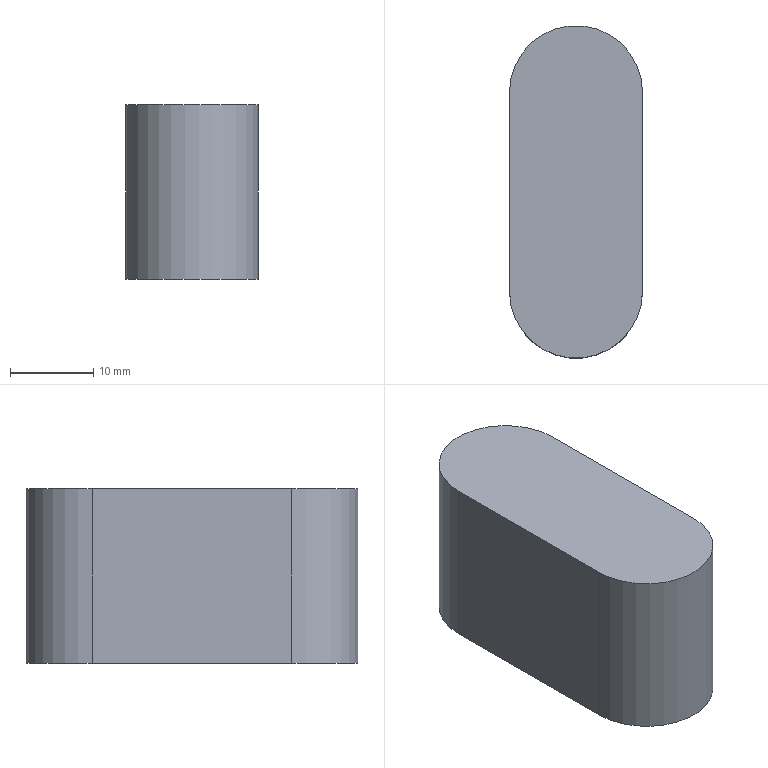Part | NX | features DATUM_CSYS 2, BLEND 1, EXTRUDE 1, OFFSET_REGION 1, SKETCH 1 | 1 solid | 6 faces | box 16 x 40 x 21 mm | volume 12286 mm3 | plane 4 | cylinder 2 | commonest cylinder face diameters 16 x2
STEP:
#1=CARTESIAN_POINT('',(-8.,12.,21.));
#2=VERTEX_POINT('',#1);
#3=CARTESIAN_POINT('',(-8.,-12.,21.));
#4=VERTEX_POINT('',#3);
#5=CARTESIAN_POINT('',(-8.,20.,21.));
#6=DIRECTION('',(0.,-1.,0.));
#7=VECTOR('',#6,1000.);
#8=LINE('',#5,#7);
#9=EDGE_CURVE('',#2,#4,#8,.T.);
#10=ORIENTED_EDGE('',*,*,#9,.F.);
#11=CARTESIAN_POINT('',(-8.,12.,0.));
#12=VERTEX_POINT('',#11);
#13=CARTESIAN_POINT('',(-8.,12.,12.));
#14=DIRECTION('',(0.,0.,-1.));
#15=VECTOR('',#14,1000.);
#16=LINE('',#13,#15);
#17=EDGE_CURVE('',#2,#12,#16,.T.);
#18=ORIENTED_EDGE('',*,*,#17,.T.);
#19=CARTESIAN_POINT('',(-8.,-12.,0.));
#20=VERTEX_POINT('',#19);
#21=CARTESIAN_POINT('',(-8.,20.,0.));
#22=DIRECTION('',(0.,-1.,0.));
#23=VECTOR('',#22,1000.);
#24=LINE('',#21,#23);
#25=EDGE_CURVE('',#12,#20,#24,.T.);
#26=ORIENTED_EDGE('',*,*,#25,.T.);
#27=CARTESIAN_POINT('',(-8.,-12.,12.));
#28=DIRECTION('',(0.,0.,-1.));
#29=VECTOR('',#28,1000.);
#30=LINE('',#27,#29);
#31=EDGE_CURVE('',#20,#4,#30,.F.);
#32=ORIENTED_EDGE('',*,*,#31,.T.);
#33=EDGE_LOOP('',(#10,#18,#26,#32));
#34=FACE_BOUND('',#33,.T.);
#35=CARTESIAN_POINT('',(-8.,20.,12.));
#36=DIRECTION('',(1.,0.,0.));
#37=DIRECTION('',(0.,0.,-1.));
#38=AXIS2_PLACEMENT_3D('',#35,#36,#37);
#39=PLANE('',#38);
#40=ADVANCED_FACE('',(#34),#39,.F.);
#41=CARTESIAN_POINT('',(8.,-12.,0.));
#42=VERTEX_POINT('',#41);
#43=CARTESIAN_POINT('',(8.,12.,0.));
#44=VERTEX_POINT('',#43);
#45=CARTESIAN_POINT('',(8.,-20.,0.));
#46=DIRECTION('',(0.,1.,0.));
#47=VECTOR('',#46,1000.);
#48=LINE('',#45,#47);
#49=EDGE_CURVE('',#42,#44,#48,.T.);
#50=ORIENTED_EDGE('',*,*,#49,.T.);
#51=CARTESIAN_POINT('',(8.,12.,21.));
#52=VERTEX_POINT('',#51);
#53=CARTESIAN_POINT('',(8.,12.,12.));
#54=DIRECTION('',(0.,0.,-1.));
#55=VECTOR('',#54,1000.);
#56=LINE('',#53,#55);
#57=EDGE_CURVE('',#44,#52,#56,.F.);
#58=ORIENTED_EDGE('',*,*,#57,.T.);
#59=CARTESIAN_POINT('',(8.,-12.,21.));
#60=VERTEX_POINT('',#59);
#61=CARTESIAN_POINT('',(8.,-20.,21.));
#62=DIRECTION('',(0.,1.,0.));
#63=VECTOR('',#62,1000.);
#64=LINE('',#61,#63);
#65=EDGE_CURVE('',#60,#52,#64,.T.);
#66=ORIENTED_EDGE('',*,*,#65,.F.);
#67=CARTESIAN_POINT('',(8.,-12.,12.));
#68=DIRECTION('',(0.,0.,-1.));
#69=VECTOR('',#68,1000.);
#70=LINE('',#67,#69);
#71=EDGE_CURVE('',#60,#42,#70,.T.);
#72=ORIENTED_EDGE('',*,*,#71,.T.);
#73=EDGE_LOOP('',(#50,#58,#66,#72));
#74=FACE_BOUND('',#73,.T.);
#75=CARTESIAN_POINT('',(8.,-20.,12.));
#76=DIRECTION('',(-1.,0.,0.));
#77=DIRECTION('',(0.,0.,1.));
#78=AXIS2_PLACEMENT_3D('',#75,#76,#77);
#79=PLANE('',#78);
#80=ADVANCED_FACE('',(#74),#79,.F.);
#81=CARTESIAN_POINT('',(0.,12.,21.));
#82=DIRECTION('',(0.,0.,1.));
#83=DIRECTION('',(1.,0.,0.));
#84=AXIS2_PLACEMENT_3D('',#81,#82,#83);
#85=CIRCLE('',#84,8.);
#86=EDGE_CURVE('',#52,#2,#85,.T.);
#87=ORIENTED_EDGE('',*,*,#86,.T.);
#88=ORIENTED_EDGE('',*,*,#9,.T.);
#89=CARTESIAN_POINT('',(0.,-12.,21.));
#90=DIRECTION('',(0.,0.,1.));
#91=DIRECTION('',(1.,0.,0.));
#92=AXIS2_PLACEMENT_3D('',#89,#90,#91);
#93=CIRCLE('',#92,8.);
#94=EDGE_CURVE('',#4,#60,#93,.T.);
#95=ORIENTED_EDGE('',*,*,#94,.T.);
#96=ORIENTED_EDGE('',*,*,#65,.T.);
#97=EDGE_LOOP('',(#87,#88,#95,#96));
#98=FACE_BOUND('',#97,.T.);
#99=CARTESIAN_POINT('',(0.,0.,21.));
#100=DIRECTION('',(0.,0.,1.));
#101=DIRECTION('',(1.,0.,0.));
#102=AXIS2_PLACEMENT_3D('',#99,#100,#101);
#103=PLANE('',#102);
#104=ADVANCED_FACE('',(#98),#103,.T.);
#105=ORIENTED_EDGE('',*,*,#25,.F.);
#106=CARTESIAN_POINT('',(0.,12.,0.));
#107=DIRECTION('',(0.,0.,1.));
#108=DIRECTION('',(1.,0.,0.));
#109=AXIS2_PLACEMENT_3D('',#106,#107,#108);
#110=CIRCLE('',#109,8.);
#111=EDGE_CURVE('',#12,#44,#110,.F.);
#112=ORIENTED_EDGE('',*,*,#111,.T.);
#113=ORIENTED_EDGE('',*,*,#49,.F.);
#114=CARTESIAN_POINT('',(0.,-12.,0.));
#115=DIRECTION('',(0.,0.,1.));
#116=DIRECTION('',(1.,0.,0.));
#117=AXIS2_PLACEMENT_3D('',#114,#115,#116);
#118=CIRCLE('',#117,8.);
#119=EDGE_CURVE('',#42,#20,#118,.F.);
#120=ORIENTED_EDGE('',*,*,#119,.T.);
#121=EDGE_LOOP('',(#105,#112,#113,#120));
#122=FACE_BOUND('',#121,.T.);
#123=CARTESIAN_POINT('',(0.,0.,0.));
#124=DIRECTION('',(0.,0.,1.));
#125=DIRECTION('',(1.,0.,0.));
#126=AXIS2_PLACEMENT_3D('',#123,#124,#125);
#127=PLANE('',#126);
#128=ADVANCED_FACE('',(#122),#127,.F.);
#129=ORIENTED_EDGE('',*,*,#111,.F.);
#130=ORIENTED_EDGE('',*,*,#17,.F.);
#131=ORIENTED_EDGE('',*,*,#86,.F.);
#132=ORIENTED_EDGE('',*,*,#57,.F.);
#133=EDGE_LOOP('',(#129,#130,#131,#132));
#134=FACE_BOUND('',#133,.T.);
#135=CARTESIAN_POINT('',(0.,12.,12.));
#136=DIRECTION('',(0.,0.,-1.));
#137=DIRECTION('',(-1.,0.,0.));
#138=AXIS2_PLACEMENT_3D('',#135,#136,#137);
#139=CYLINDRICAL_SURFACE('',#138,8.);
#140=ADVANCED_FACE('',(#134),#139,.T.);
#141=ORIENTED_EDGE('',*,*,#71,.F.);
#142=ORIENTED_EDGE('',*,*,#94,.F.);
#143=ORIENTED_EDGE('',*,*,#31,.F.);
#144=ORIENTED_EDGE('',*,*,#119,.F.);
#145=EDGE_LOOP('',(#141,#142,#143,#144));
#146=FACE_BOUND('',#145,.T.);
#147=CARTESIAN_POINT('',(0.,-12.,12.));
#148=DIRECTION('',(0.,0.,-1.));
#149=DIRECTION('',(-1.,0.,0.));
#150=AXIS2_PLACEMENT_3D('',#147,#148,#149);
#151=CYLINDRICAL_SURFACE('',#150,8.);
#152=ADVANCED_FACE('',(#146),#151,.T.);
#153=CLOSED_SHELL('',(#40,#80,#104,#128,#140,#152));
#154=MANIFOLD_SOLID_BREP('',#153);
#155=(LENGTH_UNIT()NAMED_UNIT(*)SI_UNIT(.MILLI.,.METRE.));
#156=UNCERTAINTY_MEASURE_WITH_UNIT(LENGTH_MEASURE(0.00001),#155,'','');
#157=(NAMED_UNIT(*)PLANE_ANGLE_UNIT()SI_UNIT($,.RADIAN.));
#158=(NAMED_UNIT(*)SI_UNIT($,.STERADIAN.)SOLID_ANGLE_UNIT());
#159=(GEOMETRIC_REPRESENTATION_CONTEXT(3)GLOBAL_UNCERTAINTY_ASSIGNED_CONTEXT((#156))GLOBAL_UNIT_ASSIGNED_CONTEXT((#155,#157,#158))REPRESENTATION_CONTEXT('',''));
#160=ADVANCED_BREP_SHAPE_REPRESENTATION('',(#154),#159);